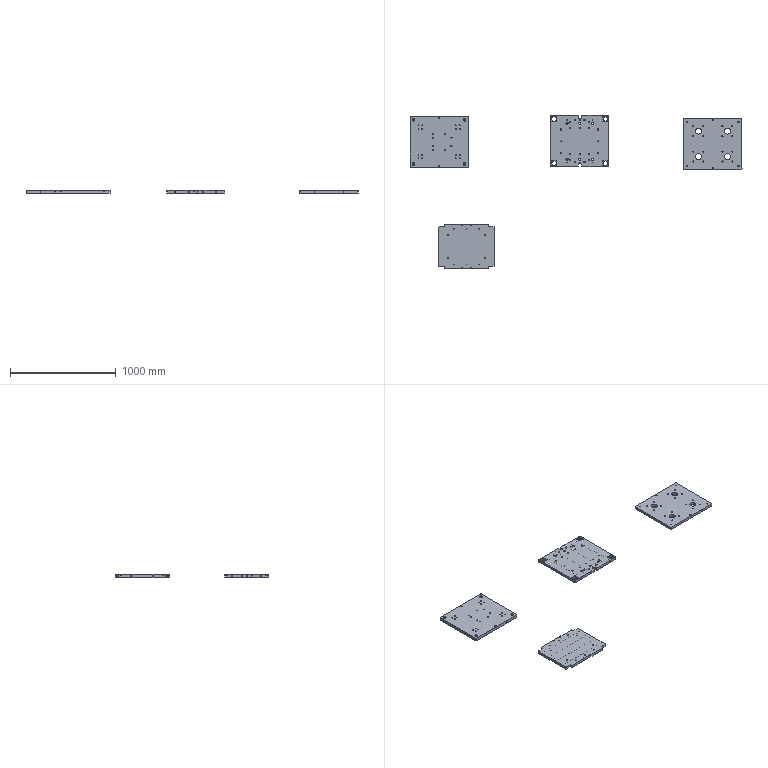NC program | Mastercam | posted with a generic post | part box 3140 x 1452 x 30 mm
Lines 1 to 1913 of 6493, first 1630 of 1913 lines:
%
O0000()
(MATERIAL - ALUMINUM MM - 2024)
( T16 | 16 FEM | H16 | XY STOCK TO LEAVE - .1 | Z STOCK TO LEAVE - .05 )
( T12 | 12 FEM | H12 | XY STOCK TO LEAVE - 0. | Z STOCK TO LEAVE - .05 )
( T7 | 4 CHM | H7 )
( T1 | 11 DR | H1 )
( T2 | 5.5 DR | H2 )
( T3 | 10.5 DR | H3 )
( T5 | 5 FEM | H5 | XY STOCK TO LEAVE - .07 | Z STOCK TO LEAVE - .05 )
( T8 | 8 FEM | H8 | XY STOCK TO LEAVE - .07 | Z STOCK TO LEAVE - .05 )
( T15 | 5.2 DR | H15 )
N100 G21
N110 G0 G17 G40 G49 G80 G90
( ? )
N120 T16 M6
N130 G0 G90 G54 X283.1 Y253.5 A0. S6000 M3
N140 G43 H16 Z50. M8
N150 Z1.2
N160 G1 Z-.294 F600.
N170 Y237.5 F4000.
N180 Y-237.5
N190 Y-253.5
N200 Z-.789 F600.
N210 Y-237.5 F4000.
N220 Y237.5
N230 Y253.5
N240 Z-1.283 F600.
N250 Y237.5 F4000.
N260 Y-237.5
N270 Y-253.5
N280 Z-1.777 F600.
N290 Y-237.5 F4000.
N300 Y237.5
N310 Y253.5
N320 Z-2.271 F600.
N330 Y237.5 F4000.
N340 Y-237.5
N350 Y-253.5
N360 Z-2.766 F600.
N370 Y-237.5 F4000.
N380 Y237.5
N390 Y253.5
N400 Z-3.26 F600.
N410 Y237.5 F4000.
N420 Y-237.5
N430 Y-253.5
N440 Z-3.754 F600.
N450 Y-237.5 F4000.
N460 Y237.5
N470 Y253.5
N480 Z-4.248 F600.
N490 Y237.5 F4000.
N500 Y-237.5
N510 Y-253.5
N520 Z-4.743 F600.
N530 Y-237.5 F4000.
N540 Y237.5
N550 Y253.5
N560 Z-5.237 F600.
N570 Y237.5 F4000.
N580 Y-237.5
N590 Y-253.5
N600 Z-5.731 F600.
N610 Y-237.5 F4000.
N620 Y237.5
N630 Y253.5
N640 Z-6.225 F600.
N650 Y237.5 F4000.
N660 Y-237.5
N670 Y-253.5
N680 Z-6.72 F600.
N690 Y-237.5 F4000.
N700 Y237.5
N710 Y253.5
N720 Z-7.214 F600.
N730 Y237.5 F4000.
N740 Y-237.5
N750 Y-253.5
N760 Z-7.708 F600.
N770 Y-237.5 F4000.
N780 Y237.5
N790 Y253.5
N800 Z-8.202 F600.
N810 Y237.5 F4000.
N820 Y-237.5
N830 Y-253.5
N840 Z-8.697 F600.
N850 Y-237.5 F4000.
N860 Y237.5
N870 Y253.5
N880 Z-9.191 F600.
N890 Y237.5 F4000.
N900 Y-237.5
N910 Y-253.5
N920 Z-9.685 F600.
N930 Y-237.5 F4000.
N940 Y237.5
N950 Y253.5
N960 Z-10.18 F600.
N970 Y237.5 F4000.
N980 Y-237.5
N990 Y-253.5
N1000 Z-10.674 F600.
N1010 Y-237.5 F4000.
N1020 Y237.5
N1030 Y253.5
N1040 Z-11.168 F600.
N1050 Y237.5 F4000.
N1060 Y-237.5
N1070 Y-253.5
N1080 Z-11.662 F600.
N1090 Y-237.5 F4000.
N1100 Y237.5
N1110 Y253.5
N1120 Z-12.157 F600.
N1130 Y237.5 F4000.
N1140 Y-237.5
N1150 Y-253.5
N1160 Z-12.651 F600.
N1170 Y-237.5 F4000.
N1180 Y237.5
N1190 Y253.5
N1200 Z-13.145 F600.
N1210 Y237.5 F4000.
N1220 Y-237.5
N1230 Y-253.5
N1240 Z-13.639 F600.
N1250 Y-237.5 F4000.
N1260 Y237.5
N1270 Y253.5
N1280 Z-14.134 F600.
N1290 Y237.5 F4000.
N1300 Y-237.5
N1310 Y-253.5
N1320 Z-14.628 F600.
N1330 Y-237.5 F4000.
N1340 Y237.5
N1350 Y253.5
N1360 Z-15.122 F600.
N1370 Y237.5 F4000.
N1380 Y-237.5
N1390 Y-253.5
N1400 Z-15.616 F600.
N1410 Y-237.5 F4000.
N1420 Y237.5
N1430 Y253.5
N1440 Z-16.111 F600.
N1450 Y237.5 F4000.
N1460 Y-237.5
N1470 Y-253.5
N1480 Z-16.605 F600.
N1490 Y-237.5 F4000.
N1500 Y237.5
N1510 Y253.5
N1520 Z-17.099 F600.
N1530 Y237.5 F4000.
N1540 Y-237.5
N1550 Y-253.5
N1560 Z-17.593 F600.
N1570 Y-237.5 F4000.
N1580 Y237.5
N1590 Y253.5
N1600 Z-18.088 F600.
N1610 Y237.5 F4000.
N1620 Y-237.5
N1630 Y-253.5
N1640 Z-18.582 F600.
N1650 Y-237.5 F4000.
N1660 Y237.5
N1670 Y253.5
N1680 Z-19.076 F600.
N1690 Y237.5 F4000.
N1700 Y-237.5
N1710 Y-253.5
N1720 Z-19.57 F600.
N1730 Y-237.5 F4000.
N1740 Y237.5
N1750 Y253.5
N1760 Z-20.065 F600.
N1770 Y237.5 F4000.
N1780 Y-237.5
N1790 Y-253.5
N1800 Z-20.559 F600.
N1810 Y-237.5 F4000.
N1820 Y237.5
N1830 Y253.5
N1840 Z-21.053 F600.
N1850 Y237.5 F4000.
N1860 Y-237.5
N1870 Y-253.5
N1880 Z-21.548 F600.
N1890 Y-237.5 F4000.
N1900 Y237.5
N1910 Y253.5
N1920 Z-22.042 F600.
N1930 Y237.5 F4000.
N1940 Y-237.5
N1950 Y-253.5
N1960 Z-22.536 F600.
N1970 Y-237.5 F4000.
N1980 Y237.5
N1990 Y253.5
N2000 Z-23.03 F600.
N2010 Y237.5 F4000.
N2020 Y-237.5
N2030 Y-253.5
N2040 Z-23.525 F600.
N2050 Y-237.5 F4000.
N2060 Y237.5
N2070 Y253.5
N2080 Z-24.019 F600.
N2090 Y237.5 F4000.
N2100 Y-237.5
N2110 Y-253.5
N2120 Z-24.513 F600.
N2130 Y-237.5 F4000.
N2140 Y237.5
N2150 Y253.5
N2160 Z-25.007 F600.
N2170 Y237.5 F4000.
N2180 Y-237.5
N2190 Y-253.5
N2200 Z-25.502 F600.
N2210 Y-237.5 F4000.
N2220 Y237.5
N2230 Y253.5
N2240 Z-25.996 F600.
N2250 Y237.5 F4000.
N2260 Y-237.5
N2270 Y-253.5
N2280 Z-26.49 F600.
N2290 Y-237.5 F4000.
N2300 Y237.5
N2310 Y253.5
N2320 Z-26.984 F600.
N2330 Y237.5 F4000.
N2340 Y-237.5
N2350 Y-253.5
N2360 Z-27.479 F600.
N2370 Y-237.5 F4000.
N2380 Y237.5
N2390 Y253.5
N2400 Z-27.973 F600.
N2410 Y237.5 F4000.
N2420 Y-237.5
N2430 Y-253.5
N2440 Z-28.467 F600.
N2450 Y-237.5 F4000.
N2460 Y237.5
N2470 Y253.5
N2480 Z-28.961 F600.
N2490 Y237.5 F4000.
N2500 Y-237.5
N2510 Y-253.5
N2520 Z-29.456 F600.
N2530 Y-237.5 F4000.
N2540 Y237.5
N2550 Y253.5
N2560 Z-29.95 F600.
N2570 Y237.5 F4000.
N2580 Y-237.5
N2590 Y-253.5
N2600 G0 Z50.
N2610 X-283.1
N2620 Z1.2
N2630 G1 Z-.294 F600.
N2640 Y-237.5 F4000.
N2650 Y237.5
N2660 Y253.5
N2670 Z-.789 F600.
N2680 Y237.5 F4000.
N2690 Y-237.5
N2700 Y-253.5
N2710 Z-1.283 F600.
N2720 Y-237.5 F4000.
N2730 Y237.5
N2740 Y253.5
N2750 Z-1.777 F600.
N2760 Y237.5 F4000.
N2770 Y-237.5
N2780 Y-253.5
N2790 Z-2.271 F600.
N2800 Y-237.5 F4000.
N2810 Y237.5
N2820 Y253.5
N2830 Z-2.766 F600.
N2840 Y237.5 F4000.
N2850 Y-237.5
N2860 Y-253.5
N2870 Z-3.26 F600.
N2880 Y-237.5 F4000.
N2890 Y237.5
N2900 Y253.5
N2910 Z-3.754 F600.
N2920 Y237.5 F4000.
N2930 Y-237.5
N2940 Y-253.5
N2950 Z-4.248 F600.
N2960 Y-237.5 F4000.
N2970 Y237.5
N2980 Y253.5
N2990 Z-4.743 F600.
N3000 Y237.5 F4000.
N3010 Y-237.5
N3020 Y-253.5
N3030 Z-5.237 F600.
N3040 Y-237.5 F4000.
N3050 Y237.5
N3060 Y253.5
N3070 Z-5.731 F600.
N3080 Y237.5 F4000.
N3090 Y-237.5
N3100 Y-253.5
N3110 Z-6.225 F600.
N3120 Y-237.5 F4000.
N3130 Y237.5
N3140 Y253.5
N3150 Z-6.72 F600.
N3160 Y237.5 F4000.
N3170 Y-237.5
N3180 Y-253.5
N3190 Z-7.214 F600.
N3200 Y-237.5 F4000.
N3210 Y237.5
N3220 Y253.5
N3230 Z-7.708 F600.
N3240 Y237.5 F4000.
N3250 Y-237.5
N3260 Y-253.5
N3270 Z-8.202 F600.
N3280 Y-237.5 F4000.
N3290 Y237.5
N3300 Y253.5
N3310 Z-8.697 F600.
N3320 Y237.5 F4000.
N3330 Y-237.5
N3340 Y-253.5
N3350 Z-9.191 F600.
N3360 Y-237.5 F4000.
N3370 Y237.5
N3380 Y253.5
N3390 Z-9.685 F600.
N3400 Y237.5 F4000.
N3410 Y-237.5
N3420 Y-253.5
N3430 Z-10.18 F600.
N3440 Y-237.5 F4000.
N3450 Y237.5
N3460 Y253.5
N3470 Z-10.674 F600.
N3480 Y237.5 F4000.
N3490 Y-237.5
N3500 Y-253.5
N3510 Z-11.168 F600.
N3520 Y-237.5 F4000.
N3530 Y237.5
N3540 Y253.5
N3550 Z-11.662 F600.
N3560 Y237.5 F4000.
N3570 Y-237.5
N3580 Y-253.5
N3590 Z-12.157 F600.
N3600 Y-237.5 F4000.
N3610 Y237.5
N3620 Y253.5
N3630 Z-12.651 F600.
N3640 Y237.5 F4000.
N3650 Y-237.5
N3660 Y-253.5
N3670 Z-13.145 F600.
N3680 Y-237.5 F4000.
N3690 Y237.5
N3700 Y253.5
N3710 Z-13.639 F600.
N3720 Y237.5 F4000.
N3730 Y-237.5
N3740 Y-253.5
N3750 Z-14.134 F600.
N3760 Y-237.5 F4000.
N3770 Y237.5
N3780 Y253.5
N3790 Z-14.628 F600.
N3800 Y237.5 F4000.
N3810 Y-237.5
N3820 Y-253.5
N3830 Z-15.122 F600.
N3840 Y-237.5 F4000.
N3850 Y237.5
N3860 Y253.5
N3870 Z-15.616 F600.
N3880 Y237.5 F4000.
N3890 Y-237.5
N3900 Y-253.5
N3910 Z-16.111 F600.
N3920 Y-237.5 F4000.
N3930 Y237.5
N3940 Y253.5
N3950 Z-16.605 F600.
N3960 Y237.5 F4000.
N3970 Y-237.5
N3980 Y-253.5
N3990 Z-17.099 F600.
N4000 Y-237.5 F4000.
N4010 Y237.5
N4020 Y253.5
N4030 Z-17.593 F600.
N4040 Y237.5 F4000.
N4050 Y-237.5
N4060 Y-253.5
N4070 Z-18.088 F600.
N4080 Y-237.5 F4000.
N4090 Y237.5
N4100 Y253.5
N4110 Z-18.582 F600.
N4120 Y237.5 F4000.
N4130 Y-237.5
N4140 Y-253.5
N4150 Z-19.076 F600.
N4160 Y-237.5 F4000.
N4170 Y237.5
N4180 Y253.5
N4190 Z-19.57 F600.
N4200 Y237.5 F4000.
N4210 Y-237.5
N4220 Y-253.5
N4230 Z-20.065 F600.
N4240 Y-237.5 F4000.
N4250 Y237.5
N4260 Y253.5
N4270 Z-20.559 F600.
N4280 Y237.5 F4000.
N4290 Y-237.5
N4300 Y-253.5
N4310 Z-21.053 F600.
N4320 Y-237.5 F4000.
N4330 Y237.5
N4340 Y253.5
N4350 Z-21.548 F600.
N4360 Y237.5 F4000.
N4370 Y-237.5
N4380 Y-253.5
N4390 Z-22.042 F600.
N4400 Y-237.5 F4000.
N4410 Y237.5
N4420 Y253.5
N4430 Z-22.536 F600.
N4440 Y237.5 F4000.
N4450 Y-237.5
N4460 Y-253.5
N4470 Z-23.03 F600.
N4480 Y-237.5 F4000.
N4490 Y237.5
N4500 Y253.5
N4510 Z-23.525 F600.
N4520 Y237.5 F4000.
N4530 Y-237.5
N4540 Y-253.5
N4550 Z-24.019 F600.
N4560 Y-237.5 F4000.
N4570 Y237.5
N4580 Y253.5
N4590 Z-24.513 F600.
N4600 Y237.5 F4000.
N4610 Y-237.5
N4620 Y-253.5
N4630 Z-25.007 F600.
N4640 Y-237.5 F4000.
N4650 Y237.5
N4660 Y253.5
N4670 Z-25.502 F600.
N4680 Y237.5 F4000.
N4690 Y-237.5
N4700 Y-253.5
N4710 Z-25.996 F600.
N4720 Y-237.5 F4000.
N4730 Y237.5
N4740 Y253.5
N4750 Z-26.49 F600.
N4760 Y237.5 F4000.
N4770 Y-237.5
N4780 Y-253.5
N4790 Z-26.984 F600.
N4800 Y-237.5 F4000.
N4810 Y237.5
N4820 Y253.5
N4830 Z-27.479 F600.
N4840 Y237.5 F4000.
N4850 Y-237.5
N4860 Y-253.5
N4870 Z-27.973 F600.
N4880 Y-237.5 F4000.
N4890 Y237.5
N4900 Y253.5
N4910 Z-28.467 F600.
N4920 Y237.5 F4000.
N4930 Y-237.5
N4940 Y-253.5
N4950 Z-28.961 F600.
N4960 Y-237.5 F4000.
N4970 Y237.5
N4980 Y253.5
N4990 Z-29.456 F600.
N5000 Y237.5 F4000.
N5010 Y-237.5
N5020 Y-253.5
N5030 Z-29.95 F600.
N5040 Y-237.5 F4000.
N5050 Y237.5
N5060 Y253.5
N5070 G0 Z50.
N5080 M5
N5090 G91 G28 Z0. M9
N5100 A0.
N5110 M01
N5120 T12 M6
N5130 G0 G90 G17 G54 X281. Y249.5 A0. S6000 M3
N5140 G43 H12 Z50. M8
N5150 Z1.2
N5160 G1 Z-14.875 F600.
N5170 Y237.5 F1000.
N5180 Y-237.5
N5190 Y-249.5
N5200 G0 Z50.
N5210 Y249.5
N5220 Z-13.875
N5230 G1 Z-29.95 F600.
N5240 Y237.5 F1000.
N5250 Y-237.5
N5260 Y-249.5
N5270 G0 Z50.
N5280 X-281.
N5290 Z1.2
N5300 G1 Z-14.875 F600.
N5310 Y-237.5 F1000.
N5320 Y237.5
N5330 Y249.5
N5340 G0 Z50.
N5350 Y-249.5
N5360 Z-13.875
N5370 G1 Z-29.95 F600.
N5380 Y-237.5 F1000.
N5390 Y237.5
N5400 Y249.5
N5410 G0 Z50.
N5420 M5
N5430 G91 G28 Z0. M9
N5440 A0.
N5450 M01
N5460 T7 M6
N5470 G0 G90 G17 G54 X275.65 Y243.5 A0. S6000 M3
N5480 G43 H7 Z50. M8
N5490 Z1.2
N5500 G1 Z-.75 F600.
N5510 Y237.5 F1000.
N5520 Y-237.5
N5530 Y-243.5
N5540 G0 Z50.
N5550 X-275.65
N5560 Z1.2
N5570 G1 Z-.75 F600.
N5580 Y-237.5 F1000.
N5590 Y237.5
N5600 Y243.5
N5610 G0 Z50.
N5620 M5
N5630 G91 G28 Z0. M9
N5640 A0.
N5650 M01
( ?X )
M00
N5660 T16 M6
N5670 G0 G90 G17 G54 X286.3 Y-235.9 A0. S6000 M3
N5680 G43 H16 Z50. M8
N5690 Z1.2
N5700 G1 Z-.485 F600.
N5710 X284.7 F4000.
N5720 G3 X283.1 Y-237.5 I0. J-1.6
N5730 G2 X270. Y-250.6 I-13.1 J0.
N5740 G1 X-270.
N5750 G2 X-283.1 Y-237.5 I0. J13.1
N5760 G3 X-284.7 Y-235.9 I-1.6 J0.
N5770 G1 X-286.3
N5780 Z-1.17 F600.
N5790 X-284.7 F4000.
N5800 G2 X-283.1 Y-237.5 I0. J-1.6
N5810 G3 X-270. Y-250.6 I13.1 J0.
N5820 G1 X270.
N5830 G3 X283.1 Y-237.5 I0. J13.1
N5840 G2 X284.7 Y-235.9 I1.6 J0.
N5850 G1 X286.3
N5860 Z-1.856 F600.
N5870 X284.7 F4000.
N5880 G3 X283.1 Y-237.5 I0. J-1.6
N5890 G2 X270. Y-250.6 I-13.1 J0.
N5900 G1 X-270.
N5910 G2 X-283.1 Y-237.5 I0. J13.1
N5920 G3 X-284.7 Y-235.9 I-1.6 J0.
N5930 G1 X-286.3
N5940 Z-2.541 F600.
N5950 X-284.7 F4000.
N5960 G2 X-283.1 Y-237.5 I0. J-1.6
N5970 G3 X-270. Y-250.6 I13.1 J0.
N5980 G1 X270.
N5990 G3 X283.1 Y-237.5 I0. J13.1
N6000 G2 X284.7 Y-235.9 I1.6 J0.
N6010 G1 X286.3
N6020 Z-3.226 F600.
N6030 X284.7 F4000.
N6040 G3 X283.1 Y-237.5 I0. J-1.6
N6050 G2 X270. Y-250.6 I-13.1 J0.
N6060 G1 X-270.
N6070 G2 X-283.1 Y-237.5 I0. J13.1
N6080 G3 X-284.7 Y-235.9 I-1.6 J0.
N6090 G1 X-286.3
N6100 Z-3.911 F600.
N6110 X-284.7 F4000.
N6120 G2 X-283.1 Y-237.5 I0. J-1.6
N6130 G3 X-270. Y-250.6 I13.1 J0.
N6140 G1 X270.
N6150 G3 X283.1 Y-237.5 I0. J13.1
N6160 G2 X284.7 Y-235.9 I1.6 J0.
N6170 G1 X286.3
N6180 Z-4.597 F600.
N6190 X284.7 F4000.
N6200 G3 X283.1 Y-237.5 I0. J-1.6
N6210 G2 X270. Y-250.6 I-13.1 J0.
N6220 G1 X-270.
N6230 G2 X-283.1 Y-237.5 I0. J13.1
N6240 G3 X-284.7 Y-235.9 I-1.6 J0.
N6250 G1 X-286.3
N6260 Z-5.282 F600.
N6270 X-284.7 F4000.
N6280 G2 X-283.1 Y-237.5 I0. J-1.6
N6290 G3 X-270. Y-250.6 I13.1 J0.
N6300 G1 X270.
N6310 G3 X283.1 Y-237.5 I0. J13.1
N6320 G2 X284.7 Y-235.9 I1.6 J0.
N6330 G1 X286.3
N6340 Z-5.967 F600.
N6350 X284.7 F4000.
N6360 G3 X283.1 Y-237.5 I0. J-1.6
N6370 G2 X270. Y-250.6 I-13.1 J0.
N6380 G1 X-270.
N6390 G2 X-283.1 Y-237.5 I0. J13.1
N6400 G3 X-284.7 Y-235.9 I-1.6 J0.
N6410 G1 X-286.3
N6420 Z-6.652 F600.
N6430 X-284.7 F4000.
N6440 G2 X-283.1 Y-237.5 I0. J-1.6
N6450 G3 X-270. Y-250.6 I13.1 J0.
N6460 G1 X270.
N6470 G3 X283.1 Y-237.5 I0. J13.1
N6480 G2 X284.7 Y-235.9 I1.6 J0.
N6490 G1 X286.3
N6500 Z-7.338 F600.
N6510 X284.7 F4000.
N6520 G3 X283.1 Y-237.5 I0. J-1.6
N6530 G2 X270. Y-250.6 I-13.1 J0.
N6540 G1 X-270.
N6550 G2 X-283.1 Y-237.5 I0. J13.1
N6560 G3 X-284.7 Y-235.9 I-1.6 J0.
N6570 G1 X-286.3
N6580 Z-8.023 F600.
N6590 X-284.7 F4000.
N6600 G2 X-283.1 Y-237.5 I0. J-1.6
N6610 G3 X-270. Y-250.6 I13.1 J0.
N6620 G1 X270.
N6630 G3 X283.1 Y-237.5 I0. J13.1
N6640 G2 X284.7 Y-235.9 I1.6 J0.
N6650 G1 X286.3
N6660 Z-8.708 F600.
N6670 X284.7 F4000.
N6680 G3 X283.1 Y-237.5 I0. J-1.6
N6690 G2 X270. Y-250.6 I-13.1 J0.
N6700 G1 X-270.
N6710 G2 X-283.1 Y-237.5 I0. J13.1
N6720 G3 X-284.7 Y-235.9 I-1.6 J0.
N6730 G1 X-286.3
N6740 Z-9.393 F600.
N6750 X-284.7 F4000.
N6760 G2 X-283.1 Y-237.5 I0. J-1.6
N6770 G3 X-270. Y-250.6 I13.1 J0.
N6780 G1 X270.
N6790 G3 X283.1 Y-237.5 I0. J13.1
N6800 G2 X284.7 Y-235.9 I1.6 J0.
N6810 G1 X286.3
N6820 Z-10.078 F600.
N6830 X284.7 F4000.
N6840 G3 X283.1 Y-237.5 I0. J-1.6
N6850 G2 X270. Y-250.6 I-13.1 J0.
N6860 G1 X-270.
N6870 G2 X-283.1 Y-237.5 I0. J13.1
N6880 G3 X-284.7 Y-235.9 I-1.6 J0.
N6890 G1 X-286.3
N6900 Z-10.764 F600.
N6910 X-284.7 F4000.
N6920 G2 X-283.1 Y-237.5 I0. J-1.6
N6930 G3 X-270. Y-250.6 I13.1 J0.
N6940 G1 X270.
N6950 G3 X283.1 Y-237.5 I0. J13.1
N6960 G2 X284.7 Y-235.9 I1.6 J0.
N6970 G1 X286.3
N6980 Z-11.449 F600.
N6990 X284.7 F4000.
N7000 G3 X283.1 Y-237.5 I0. J-1.6
N7010 G2 X270. Y-250.6 I-13.1 J0.
N7020 G1 X-270.
N7030 G2 X-283.1 Y-237.5 I0. J13.1
N7040 G3 X-284.7 Y-235.9 I-1.6 J0.
N7050 G1 X-286.3
N7060 Z-12.134 F600.
N7070 X-284.7 F4000.
N7080 G2 X-283.1 Y-237.5 I0. J-1.6
N7090 G3 X-270. Y-250.6 I13.1 J0.
N7100 G1 X270.
N7110 G3 X283.1 Y-237.5 I0. J13.1
N7120 G2 X284.7 Y-235.9 I1.6 J0.
N7130 G1 X286.3
N7140 Z-12.819 F600.
N7150 X284.7 F4000.
N7160 G3 X283.1 Y-237.5 I0. J-1.6
N7170 G2 X270. Y-250.6 I-13.1 J0.
N7180 G1 X-270.
N7190 G2 X-283.1 Y-237.5 I0. J13.1
N7200 G3 X-284.7 Y-235.9 I-1.6 J0.
N7210 G1 X-286.3
N7220 Z-13.505 F600.
N7230 X-284.7 F4000.
N7240 G2 X-283.1 Y-237.5 I0. J-1.6
N7250 G3 X-270. Y-250.6 I13.1 J0.
N7260 G1 X270.
N7270 G3 X283.1 Y-237.5 I0. J13.1
N7280 G2 X284.7 Y-235.9 I1.6 J0.
N7290 G1 X286.3
N7300 Z-14.19 F600.
N7310 X284.7 F4000.
N7320 G3 X283.1 Y-237.5 I0. J-1.6
N7330 G2 X270. Y-250.6 I-13.1 J0.
N7340 G1 X-270.
N7350 G2 X-283.1 Y-237.5 I0. J13.1
N7360 G3 X-284.7 Y-235.9 I-1.6 J0.
N7370 G1 X-286.3
N7380 Z-14.875 F600.
N7390 X-284.7 F4000.
N7400 G2 X-283.1 Y-237.5 I0. J-1.6
N7410 G3 X-270. Y-250.6 I13.1 J0.
N7420 G1 X270.
N7430 G3 X283.1 Y-237.5 I0. J13.1
N7440 G2 X284.7 Y-235.9 I1.6 J0.
N7450 G1 X286.3
N7460 Z-15.56 F600.
N7470 X284.7 F4000.
N7480 G3 X283.1 Y-237.5 I0. J-1.6
N7490 G2 X270. Y-250.6 I-13.1 J0.
N7500 G1 X-270.
N7510 G2 X-283.1 Y-237.5 I0. J13.1
N7520 G3 X-284.7 Y-235.9 I-1.6 J0.
N7530 G1 X-286.3
N7540 Z-16.245 F600.
N7550 X-284.7 F4000.
N7560 G2 X-283.1 Y-237.5 I0. J-1.6
N7570 G3 X-270. Y-250.6 I13.1 J0.
N7580 G1 X270.
N7590 G3 X283.1 Y-237.5 I0. J13.1
N7600 G2 X284.7 Y-235.9 I1.6 J0.
N7610 G1 X286.3
N7620 Z-16.931 F600.
N7630 X284.7 F4000.
N7640 G3 X283.1 Y-237.5 I0. J-1.6
N7650 G2 X270. Y-250.6 I-13.1 J0.
N7660 G1 X-270.
N7670 G2 X-283.1 Y-237.5 I0. J13.1
N7680 G3 X-284.7 Y-235.9 I-1.6 J0.
N7690 G1 X-286.3
N7700 Z-17.616 F600.
N7710 X-284.7 F4000.
N7720 G2 X-283.1 Y-237.5 I0. J-1.6
N7730 G3 X-270. Y-250.6 I13.1 J0.
N7740 G1 X270.
N7750 G3 X283.1 Y-237.5 I0. J13.1
N7760 G2 X284.7 Y-235.9 I1.6 J0.
N7770 G1 X286.3
N7780 Z-18.301 F600.
N7790 X284.7 F4000.
N7800 G3 X283.1 Y-237.5 I0. J-1.6
N7810 G2 X270. Y-250.6 I-13.1 J0.
N7820 G1 X-270.
N7830 G2 X-283.1 Y-237.5 I0. J13.1
N7840 G3 X-284.7 Y-235.9 I-1.6 J0.
N7850 G1 X-286.3
N7860 Z-18.986 F600.
N7870 X-284.7 F4000.
N7880 G2 X-283.1 Y-237.5 I0. J-1.6
N7890 G3 X-270. Y-250.6 I13.1 J0.
N7900 G1 X270.
N7910 G3 X283.1 Y-237.5 I0. J13.1
N7920 G2 X284.7 Y-235.9 I1.6 J0.
N7930 G1 X286.3
N7940 Z-19.672 F600.
N7950 X284.7 F4000.
N7960 G3 X283.1 Y-237.5 I0. J-1.6
N7970 G2 X270. Y-250.6 I-13.1 J0.
N7980 G1 X-270.
N7990 G2 X-283.1 Y-237.5 I0. J13.1
N8000 G3 X-284.7 Y-235.9 I-1.6 J0.
N8010 G1 X-286.3
N8020 Z-20.357 F600.
N8030 X-284.7 F4000.
N8040 G2 X-283.1 Y-237.5 I0. J-1.6
N8050 G3 X-270. Y-250.6 I13.1 J0.
N8060 G1 X270.
N8070 G3 X283.1 Y-237.5 I0. J13.1
N8080 G2 X284.7 Y-235.9 I1.6 J0.
N8090 G1 X286.3
N8100 Z-21.042 F600.
N8110 X284.7 F4000.
N8120 G3 X283.1 Y-237.5 I0. J-1.6
N8130 G2 X270. Y-250.6 I-13.1 J0.
N8140 G1 X-270.
N8150 G2 X-283.1 Y-237.5 I0. J13.1
N8160 G3 X-284.7 Y-235.9 I-1.6 J0.
N8170 G1 X-286.3
N8180 Z-21.727 F600.
N8190 X-284.7 F4000.
N8200 G2 X-283.1 Y-237.5 I0. J-1.6
N8210 G3 X-270. Y-250.6 I13.1 J0.
N8220 G1 X270.
N8230 G3 X283.1 Y-237.5 I0. J13.1
N8240 G2 X284.7 Y-235.9 I1.6 J0.
N8250 G1 X286.3
N8260 Z-22.413 F600.
N8270 X284.7 F4000.
N8280 G3 X283.1 Y-237.5 I0. J-1.6
N8290 G2 X270. Y-250.6 I-13.1 J0.
N8300 G1 X-270.
N8310 G2 X-283.1 Y-237.5 I0. J13.1
N8320 G3 X-284.7 Y-235.9 I-1.6 J0.
N8330 G1 X-286.3
N8340 Z-23.098 F600.
N8350 X-284.7 F4000.
N8360 G2 X-283.1 Y-237.5 I0. J-1.6
N8370 G3 X-270. Y-250.6 I13.1 J0.
N8380 G1 X270.
N8390 G3 X283.1 Y-237.5 I0. J13.1
N8400 G2 X284.7 Y-235.9 I1.6 J0.
N8410 G1 X286.3
N8420 Z-23.783 F600.
N8430 X284.7 F4000.
N8440 G3 X283.1 Y-237.5 I0. J-1.6
N8450 G2 X270. Y-250.6 I-13.1 J0.
N8460 G1 X-270.
N8470 G2 X-283.1 Y-237.5 I0. J13.1
N8480 G3 X-284.7 Y-235.9 I-1.6 J0.
N8490 G1 X-286.3
N8500 Z-24.468 F600.
N8510 X-284.7 F4000.
N8520 G2 X-283.1 Y-237.5 I0. J-1.6
N8530 G3 X-270. Y-250.6 I13.1 J0.
N8540 G1 X270.
N8550 G3 X283.1 Y-237.5 I0. J13.1
N8560 G2 X284.7 Y-235.9 I1.6 J0.
N8570 G1 X286.3
N8580 Z-25.153 F600.
N8590 X284.7 F4000.
N8600 G3 X283.1 Y-237.5 I0. J-1.6
N8610 G2 X270. Y-250.6 I-13.1 J0.
N8620 G1 X-270.
N8630 G2 X-283.1 Y-237.5 I0. J13.1
N8640 G3 X-284.7 Y-235.9 I-1.6 J0.
N8650 G1 X-286.3
N8660 Z-25.839 F600.
N8670 X-284.7 F4000.
N8680 G2 X-283.1 Y-237.5 I0. J-1.6
N8690 G3 X-270. Y-250.6 I13.1 J0.
N8700 G1 X270.
N8710 G3 X283.1 Y-237.5 I0. J13.1
N8720 G2 X284.7 Y-235.9 I1.6 J0.
N8730 G1 X286.3
N8740 Z-26.524 F600.
N8750 X284.7 F4000.
N8760 G3 X283.1 Y-237.5 I0. J-1.6
N8770 G2 X270. Y-250.6 I-13.1 J0.
N8780 G1 X-270.
N8790 G2 X-283.1 Y-237.5 I0. J13.1
N8800 G3 X-284.7 Y-235.9 I-1.6 J0.
N8810 G1 X-286.3
N8820 Z-27.209 F600.
N8830 X-284.7 F4000.
N8840 G2 X-283.1 Y-237.5 I0. J-1.6
N8850 G3 X-270. Y-250.6 I13.1 J0.
N8860 G1 X270.
N8870 G3 X283.1 Y-237.5 I0. J13.1
N8880 G2 X284.7 Y-235.9 I1.6 J0.
N8890 G1 X286.3
N8900 Z-27.894 F600.
N8910 X284.7 F4000.
N8920 G3 X283.1 Y-237.5 I0. J-1.6
N8930 G2 X270. Y-250.6 I-13.1 J0.
N8940 G1 X-270.
N8950 G2 X-283.1 Y-237.5 I0. J13.1
N8960 G3 X-284.7 Y-235.9 I-1.6 J0.
N8970 G1 X-286.3
N8980 Z-28.58 F600.
N8990 X-284.7 F4000.
N9000 G2 X-283.1 Y-237.5 I0. J-1.6
N9010 G3 X-270. Y-250.6 I13.1 J0.
N9020 G1 X270.
N9030 G3 X283.1 Y-237.5 I0. J13.1
N9040 G2 X284.7 Y-235.9 I1.6 J0.
N9050 G1 X286.3
N9060 Z-29.265 F600.
N9070 X284.7 F4000.
N9080 G3 X283.1 Y-237.5 I0. J-1.6
N9090 G2 X270. Y-250.6 I-13.1 J0.
N9100 G1 X-270.
N9110 G2 X-283.1 Y-237.5 I0. J13.1
N9120 G3 X-284.7 Y-235.9 I-1.6 J0.
N9130 G1 X-286.3
N9140 Z-29.95 F600.
N9150 X-284.7 F4000.
N9160 G2 X-283.1 Y-237.5 I0. J-1.6
N9170 G3 X-270. Y-250.6 I13.1 J0.
N9180 G1 X270.
N9190 G3 X283.1 Y-237.5 I0. J13.1
N9200 G2 X284.7 Y-235.9 I1.6 J0.
N9210 G1 X286.3
N9220 G0 Z50.
N9230 X-286.3 Y235.9
N9240 Z1.2
N9250 G1 Z-.485 F600.
N9260 X-284.7 F4000.
N9270 G3 X-283.1 Y237.5 I0. J1.6
N9280 G2 X-270. Y250.6 I13.1 J0.
N9290 G1 X270.
N9300 G2 X283.1 Y237.5 I0. J-13.1
N9310 G3 X284.7 Y235.9 I1.6 J0.
N9320 G1 X286.3
N9330 Z-1.17 F600.
N9340 X284.7 F4000.
N9350 G2 X283.1 Y237.5 I0. J1.6
N9360 G3 X270. Y250.6 I-13.1 J0.
N9370 G1 X-270.
N9380 G3 X-283.1 Y237.5 I0. J-13.1
N9390 G2 X-284.7 Y235.9 I-1.6 J0.
N9400 G1 X-286.3
N9410 Z-1.856 F600.
N9420 X-284.7 F4000.
N9430 G3 X-283.1 Y237.5 I0. J1.6
N9440 G2 X-270. Y250.6 I13.1 J0.
N9450 G1 X270.
N9460 G2 X283.1 Y237.5 I0. J-13.1
N9470 G3 X284.7 Y235.9 I1.6 J0.
N9480 G1 X286.3
N9490 Z-2.541 F600.
N9500 X284.7 F4000.
N9510 G2 X283.1 Y237.5 I0. J1.6
N9520 G3 X270. Y250.6 I-13.1 J0.
N9530 G1 X-270.
N9540 G3 X-283.1 Y237.5 I0. J-13.1
N9550 G2 X-284.7 Y235.9 I-1.6 J0.
N9560 G1 X-286.3
N9570 Z-3.226 F600.
N9580 X-284.7 F4000.
N9590 G3 X-283.1 Y237.5 I0. J1.6
N9600 G2 X-270. Y250.6 I13.1 J0.
N9610 G1 X270.
N9620 G2 X283.1 Y237.5 I0. J-13.1
N9630 G3 X284.7 Y235.9 I1.6 J0.
N9640 G1 X286.3
N9650 Z-3.911 F600.
N9660 X284.7 F4000.
N9670 G2 X283.1 Y237.5 I0. J1.6
N9680 G3 X270. Y250.6 I-13.1 J0.
N9690 G1 X-270.
N9700 G3 X-283.1 Y237.5 I0. J-13.1
N9710 G2 X-284.7 Y235.9 I-1.6 J0.
N9720 G1 X-286.3
N9730 Z-4.597 F600.
N9740 X-284.7 F4000.
N9750 G3 X-283.1 Y237.5 I0. J1.6
N9760 G2 X-270. Y250.6 I13.1 J0.
N9770 G1 X270.
N9780 G2 X283.1 Y237.5 I0. J-13.1
N9790 G3 X284.7 Y235.9 I1.6 J0.
N9800 G1 X286.3
N9810 Z-5.282 F600.
N9820 X284.7 F4000.
N9830 G2 X283.1 Y237.5 I0. J1.6
N9840 G3 X270. Y250.6 I-13.1 J0.
N9850 G1 X-270.
N9860 G3 X-283.1 Y237.5 I0. J-13.1
N9870 G2 X-284.7 Y235.9 I-1.6 J0.
N9880 G1 X-286.3
N9890 Z-5.967 F600.
N9900 X-284.7 F4000.
N9910 G3 X-283.1 Y237.5 I0. J1.6
N9920 G2 X-270. Y250.6 I13.1 J0.
N9930 G1 X270.
N9940 G2 X283.1 Y237.5 I0. J-13.1
N9950 G3 X284.7 Y235.9 I1.6 J0.
N9960 G1 X286.3
N9970 Z-6.652 F600.
N9980 X284.7 F4000.
N9990 G2 X283.1 Y237.5 I0. J1.6
N100 G3 X270. Y250.6 I-13.1 J0.
N110 G1 X-270.
N120 G3 X-283.1 Y237.5 I0. J-13.1
N130 G2 X-284.7 Y235.9 I-1.6 J0.
N140 G1 X-286.3
N150 Z-7.338 F600.
N160 X-284.7 F4000.
N170 G3 X-283.1 Y237.5 I0. J1.6
N180 G2 X-270. Y250.6 I13.1 J0.
N190 G1 X270.
N200 G2 X283.1 Y237.5 I0. J-13.1
N210 G3 X284.7 Y235.9 I1.6 J0.
N220 G1 X286.3
N230 Z-8.023 F600.
N240 X284.7 F4000.
N250 G2 X283.1 Y237.5 I0. J1.6
N260 G3 X270. Y250.6 I-13.1 J0.
N270 G1 X-270.
N280 G3 X-283.1 Y237.5 I0. J-13.1
N290 G2 X-284.7 Y235.9 I-1.6 J0.
N300 G1 X-286.3
N310 Z-8.708 F600.
N320 X-284.7 F4000.
N330 G3 X-283.1 Y237.5 I0. J1.6
N340 G2 X-270. Y250.6 I13.1 J0.
N350 G1 X270.
N360 G2 X283.1 Y237.5 I0. J-13.1
N370 G3 X284.7 Y235.9 I1.6 J0.
N380 G1 X286.3
N390 Z-9.393 F600.
N400 X284.7 F4000.
N410 G2 X283.1 Y237.5 I0. J1.6
N420 G3 X270. Y250.6 I-13.1 J0.
N430 G1 X-270.
N440 G3 X-283.1 Y237.5 I0. J-13.1
N450 G2 X-284.7 Y235.9 I-1.6 J0.
N460 G1 X-286.3
N470 Z-10.078 F600.
N480 X-284.7 F4000.
N490 G3 X-283.1 Y237.5 I0. J1.6
N500 G2 X-270. Y250.6 I13.1 J0.
N510 G1 X270.
N520 G2 X283.1 Y237.5 I0. J-13.1
N530 G3 X284.7 Y235.9 I1.6 J0.
N540 G1 X286.3
N550 Z-10.764 F600.
N560 X284.7 F4000.
N570 G2 X283.1 Y237.5 I0. J1.6
N580 G3 X270. Y250.6 I-13.1 J0.
N590 G1 X-270.
N600 G3 X-283.1 Y237.5 I0. J-13.1
N610 G2 X-284.7 Y235.9 I-1.6 J0.
N620 G1 X-286.3
N630 Z-11.449 F600.
N640 X-284.7 F4000.
N650 G3 X-283.1 Y237.5 I0. J1.6
N660 G2 X-270. Y250.6 I13.1 J0.
N670 G1 X270.
N680 G2 X283.1 Y237.5 I0. J-13.1
N690 G3 X284.7 Y235.9 I1.6 J0.
N700 G1 X286.3
N710 Z-12.134 F600.
N720 X284.7 F4000.
N730 G2 X283.1 Y237.5 I0. J1.6
N740 G3 X270. Y250.6 I-13.1 J0.
N750 G1 X-270.
N760 G3 X-283.1 Y237.5 I0. J-13.1
N770 G2 X-284.7 Y235.9 I-1.6 J0.
N780 G1 X-286.3
N790 Z-12.819 F600.
N800 X-284.7 F4000.
N810 G3 X-283.1 Y237.5 I0. J1.6
N820 G2 X-270. Y250.6 I13.1 J0.
N830 G1 X270.
N840 G2 X283.1 Y237.5 I0. J-13.1
N850 G3 X284.7 Y235.9 I1.6 J0.
N860 G1 X286.3
N870 Z-13.505 F600.
N880 X284.7 F4000.
N890 G2 X283.1 Y237.5 I0. J1.6
N900 G3 X270. Y250.6 I-13.1 J0.
N910 G1 X-270.
N920 G3 X-283.1 Y237.5 I0. J-13.1
N930 G2 X-284.7 Y235.9 I-1.6 J0.
N940 G1 X-286.3
N950 Z-14.19 F600.
N960 X-284.7 F4000.
N970 G3 X-283.1 Y237.5 I0. J1.6
N980 G2 X-270. Y250.6 I13.1 J0.
N990 G1 X270.
N1000 G2 X283.1 Y237.5 I0. J-13.1
N1010 G3 X284.7 Y235.9 I1.6 J0.
N1020 G1 X286.3
N1030 Z-14.875 F600.
N1040 X284.7 F4000.
N1050 G2 X283.1 Y237.5 I0. J1.6
N1060 G3 X270. Y250.6 I-13.1 J0.
N1070 G1 X-270.
N1080 G3 X-283.1 Y237.5 I0. J-13.1
N1090 G2 X-284.7 Y235.9 I-1.6 J0.
N1100 G1 X-286.3
N1110 Z-15.56 F600.
N1120 X-284.7 F4000.
N1130 G3 X-283.1 Y237.5 I0. J1.6
N1140 G2 X-270. Y250.6 I13.1 J0.
N1150 G1 X270.
N1160 G2 X283.1 Y237.5 I0. J-13.1
N1170 G3 X284.7 Y235.9 I1.6 J0.
N1180 G1 X286.3
N1190 Z-16.245 F600.
N1200 X284.7 F4000.
N1210 G2 X283.1 Y237.5 I0. J1.6
N1220 G3 X270. Y250.6 I-13.1 J0.
N1230 G1 X-270.
N1240 G3 X-283.1 Y237.5 I0. J-13.1
N1250 G2 X-284.7 Y235.9 I-1.6 J0.
N1260 G1 X-286.3
N1270 Z-16.931 F600.
N1280 X-284.7 F4000.
N1290 G3 X-283.1 Y237.5 I0. J1.6
N1300 G2 X-270. Y250.6 I13.1 J0.
N1310 G1 X270.
N1320 G2 X283.1 Y237.5 I0. J-13.1
N1330 G3 X284.7 Y235.9 I1.6 J0.
N1340 G1 X286.3
N1350 Z-17.616 F600.
N1360 X284.7 F4000.
N1370 G2 X283.1 Y237.5 I0. J1.6
N1380 G3 X270. Y250.6 I-13.1 J0.
N1390 G1 X-270.
N1400 G3 X-283.1 Y237.5 I0. J-13.1
N1410 G2 X-284.7 Y235.9 I-1.6 J0.
N1420 G1 X-286.3
N1430 Z-18.301 F600.
N1440 X-284.7 F4000.
N1450 G3 X-283.1 Y237.5 I0. J1.6
N1460 G2 X-270. Y250.6 I13.1 J0.
N1470 G1 X270.
N1480 G2 X283.1 Y237.5 I0. J-13.1
N1490 G3 X284.7 Y235.9 I1.6 J0.
N1500 G1 X286.3
N1510 Z-18.986 F600.
N1520 X284.7 F4000.
N1530 G2 X283.1 Y237.5 I0. J1.6
N1540 G3 X270. Y250.6 I-13.1 J0.
N1550 G1 X-270.
N1560 G3 X-283.1 Y237.5 I0. J-13.1
N1570 G2 X-284.7 Y235.9 I-1.6 J0.
N1580 G1 X-286.3
N1590 Z-19.672 F600.
N1600 X-284.7 F4000.
N1610 G3 X-283.1 Y237.5 I0. J1.6
N1620 G2 X-270. Y250.6 I13.1 J0.
N1630 G1 X270.
N1640 G2 X283.1 Y237.5 I0. J-13.1
N1650 G3 X284.7 Y235.9 I1.6 J0.
N1660 G1 X286.3
N1670 Z-20.357 F600.
N1680 X284.7 F4000.
N1690 G2 X283.1 Y237.5 I0. J1.6
N1700 G3 X270. Y250.6 I-13.1 J0.
N1710 G1 X-270.
N1720 G3 X-283.1 Y237.5 I0. J-13.1
N1730 G2 X-284.7 Y235.9 I-1.6 J0.
N1740 G1 X-286.3
N1750 Z-21.042 F600.
N1760 X-284.7 F4000.
N1770 G3 X-283.1 Y237.5 I0. J1.6
N1780 G2 X-270. Y250.6 I13.1 J0.
N1790 G1 X270.
N1800 G2 X283.1 Y237.5 I0. J-13.1
N1810 G3 X284.7 Y235.9 I1.6 J0.
N1820 G1 X286.3
N1830 Z-21.727 F600.
N1840 X284.7 F4000.
N1850 G2 X283.1 Y237.5 I0. J1.6
N1860 G3 X270. Y250.6 I-13.1 J0.
N1870 G1 X-270.
N1880 G3 X-283.1 Y237.5 I0. J-13.1
N1890 G2 X-284.7 Y235.9 I-1.6 J0.
N1900 G1 X-286.3
N1910 Z-22.413 F600.
N1920 X-284.7 F4000.
N1930 G3 X-283.1 Y237.5 I0. J1.6
N1940 G2 X-270. Y250.6 I13.1 J0.
N1950 G1 X270.
N1960 G2 X283.1 Y237.5 I0. J-13.1
N1970 G3 X284.7 Y235.9 I1.6 J0.
N1980 G1 X286.3
N1990 Z-23.098 F600.
N2000 X284.7 F4000.
N2010 G2 X283.1 Y237.5 I0. J1.6
N2020 G3 X270. Y250.6 I-13.1 J0.
N2030 G1 X-270.
N2040 G3 X-283.1 Y237.5 I0. J-13.1
N2050 G2 X-284.7 Y235.9 I-1.6 J0.
N2060 G1 X-286.3
N2070 Z-23.783 F600.
N2080 X-284.7 F4000.
N2090 G3 X-283.1 Y237.5 I0. J1.6
N2100 G2 X-270. Y250.6 I13.1 J0.
N2110 G1 X270.
N2120 G2 X283.1 Y237.5 I0. J-13.1
N2130 G3 X284.7 Y235.9 I1.6 J0.
N2140 G1 X286.3
N2150 Z-24.468 F600.
N2160 X284.7 F4000.
N2170 G2 X283.1 Y237.5 I0. J1.6
N2180 G3 X270. Y250.6 I-13.1 J0.
N2190 G1 X-270.
N2200 G3 X-283.1 Y237.5 I0. J-13.1
N2210 G2 X-284.7 Y235.9 I-1.6 J0.
N2220 G1 X-286.3
N2230 Z-25.153 F600.
N2240 X-284.7 F4000.
N2250 G3 X-283.1 Y237.5 I0. J1.6
N2260 G2 X-270. Y250.6 I13.1 J0.
N2270 G1 X270.
N2280 G2 X283.1 Y237.5 I0. J-13.1
N2290 G3 X284.7 Y235.9 I1.6 J0.
N2300 G1 X286.3
N2310 Z-25.839 F600.
N2320 X284.7 F4000.
N2330 G2 X283.1 Y237.5 I0. J1.6
N2340 G3 X270. Y250.6 I-13.1 J0.
N2350 G1 X-270.
N2360 G3 X-283.1 Y237.5 I0. J-13.1
N2370 G2 X-284.7 Y235.9 I-1.6 J0.
N2380 G1 X-286.3
N2390 Z-26.524 F600.
N2400 X-284.7 F4000.
N2410 G3 X-283.1 Y237.5 I0. J1.6
N2420 G2 X-270. Y250.6 I13.1 J0.
N2430 G1 X270.
N2440 G2 X283.1 Y237.5 I0. J-13.1
N2450 G3 X284.7 Y235.9 I1.6 J0.
N2460 G1 X286.3
N2470 Z-27.209 F600.
N2480 X284.7 F4000.
N2490 G2 X283.1 Y237.5 I0. J1.6
N2500 G3 X270. Y250.6 I-13.1 J0.
N2510 G1 X-270.
N2520 G3 X-283.1 Y237.5 I0. J-13.1
N2530 G2 X-284.7 Y235.9 I-1.6 J0.
N2540 G1 X-286.3
N2550 Z-27.894 F600.
N2560 X-284.7 F4000.
N2570 G3 X-283.1 Y237.5 I0. J1.6
N2580 G2 X-270. Y250.6 I13.1 J0.
N2590 G1 X270.
N2600 G2 X283.1 Y237.5 I0. J-13.1
N2610 G3 X284.7 Y235.9 I1.6 J0.
N2620 G1 X286.3
N2630 Z-28.58 F600.
N2640 X284.7 F4000.
N2650 G2 X283.1 Y237.5 I0. J1.6
N2660 G3 X270. Y250.6 I-13.1 J0.
N2670 G1 X-270.
N2680 G3 X-283.1 Y237.5 I0. J-13.1
N2690 G2 X-284.7 Y235.9 I-1.6 J0.
N2700 G1 X-286.3
N2710 Z-29.265 F600.
N2720 X-284.7 F4000.
N2730 G3 X-283.1 Y237.5 I0. J1.6
N2740 G2 X-270. Y250.6 I13.1 J0.
N2750 G1 X270.
N2760 G2 X283.1 Y237.5 I0. J-13.1
N2770 G3 X284.7 Y235.9 I1.6 J0.
N2780 G1 X286.3
N2790 Z-29.95 F600.
N2800 X284.7 F4000.
N2810 G2 X283.1 Y237.5 I0. J1.6
N2820 G3 X270. Y250.6 I-13.1 J0.
N2830 G1 X-270.
N2840 G3 X-283.1 Y237.5 I0. J-13.1
N2850 G2 X-284.7 Y235.9 I-1.6 J0.
N2860 G1 X-286.3
N2870 G0 Z50.
N2880 M5
N2890 G91 G28 Z0. M9
N2900 A0.
N2910 M01
N2920 T12 M6
N2930 G0 G90 G17 G54 X283.4 Y-236.3 A0. S6000 M3
N2940 G43 H12 Z50. M8
N2950 Z1.2
N2960 G1 Z-14.875 F600.
N2970 X282.2 F1000.
N2980 G3 X281. Y-237.5 I0. J-1.2
N2990 G2 X270. Y-248.5 I-11. J0.
N3000 G1 X-270.
N3010 G2 X-281. Y-237.5 I0. J11.
N3020 G3 X-282.2 Y-236.3 I-1.2 J0.
N3030 G1 X-283.4
N3040 G0 Z50.
N3050 X283.4
N3060 Z-13.875
N3070 G1 Z-29.95 F600.
N3080 X282.2 F1000.
N3090 G3 X281. Y-237.5 I0. J-1.2
N3100 G2 X270. Y-248.5 I-11. J0.
N3110 G1 X-270.
N3120 G2 X-281. Y-237.5 I0. J11.
N3130 G3 X-282.2 Y-236.3 I-1.2 J0.
N3140 G1 X-283.4
N3150 G0 Z50.
N3160 Y236.3
N3170 Z1.2
N3180 G1 Z-14.875 F600.
N3190 X-282.2 F1000.
N3200 G3 X-281. Y237.5 I0. J1.2
N3210 G2 X-270. Y248.5 I11. J0.
N3220 G1 X270.
N3230 G2 X281. Y237.5 I0. J-11.
N3240 G3 X282.2 Y236.3 I1.2 J0.
N3250 G1 X283.4
N3260 G0 Z50.
N3270 X-283.4
N3280 Z-13.875
N3290 G1 Z-29.95 F600.
N3300 X-282.2 F1000.
N3310 G3 X-281. Y237.5 I0. J1.2
N3320 G2 X-270. Y248.5 I11. J0.
N3330 G1 X270.
N3340 G2 X281. Y237.5 I0. J-11.
N3350 G3 X282.2 Y236.3 I1.2 J0.
N3360 G1 X283.4
N3370 G0 Z50.
N3380 M5
N3390 G91 G28 Z0. M9
N3400 A0.
N3410 M01
N3420 T7 M6
N3430 G0 G90 G17 G54 X276.45 Y-237.1 A0. S6000 M3
N3440 G43 H7 Z50. M8
N3450 Z1.2
N3460 G1 Z-.75 F600.
N3470 X276.05 F1000.
N3480 G3 X275.65 Y-237.5 I0. J-.4
N3490 G2 X270. Y-243.15 I-5.65 J0.
N3500 G1 X-270.
N3510 G2 X-275.65 Y-237.5 I0. J5.65
N3520 G3 X-276.05 Y-237.1 I-.4 J0.
N3530 G1 X-276.45
N3540 G0 Z50.
N3550 Y237.1
N3560 Z1.2
N3570 G1 Z-.75 F600.
N3580 X-276.05 F1000.
N3590 G3 X-275.65 Y237.5 I0. J.4
N3600 G2 X-270. Y243.15 I5.65 J0.
N3610 G1 X270.
N3620 G2 X275.65 Y237.5 I0. J-5.65
N3630 G3 X276.05 Y237.1 I.4 J0.
N3640 G1 X276.45
N3650 G0 Z50.
N3660 X242. Y-209.
N3670 G98 G81 Z-.7 R1. F200.
N3680 X194.5 Y-156.
N3690 Y-124.
N3700 X158.5 Y-156.
N3710 Y-124.
N3720 X117. Y-40.
N3730 X55. Y-72.5
N3740 X-55.
N3750 X-57. Y-40.
N3760 Y40.
N3770 X-55. Y72.5
N3780 X55.
N3790 X117. Y40.
N3800 X158.5 Y124.
N3810 X194.5
N3820 Y156.
N3830 X242. Y209.
N3840 X158.5 Y156.
N3850 X0. Y227.5
N3860 X-158.5 Y156.
N3870 X-242. Y209.
N3880 X-194.5 Y156.
N3890 Y124.
N3900 X-158.5
N3910 Y-124.
N3920 X-194.5
N3930 Y-156.
N3940 X-242. Y-209.
N3950 X-158.5 Y-156.
N3960 X0. Y-227.5
N3970 G80
N3980 M5
N3990 G91 G0 G28 Z0. M9
N4000 A0.
N4010 M01
N4020 T1 M6
N4030 G0 G90 G17 G54 X242. Y-209. A0. S800 M3
N4040 G43 H1 Z50. M8
N4050 G98 G83 Z-29.8 R1. Q2. F60.
N4060 X0. Y-227.5
N4070 X-242. Y-209.
N4080 Y209.
N4090 X0. Y227.5
N4100 X242. Y209.
N4110 G80
N4120 M5
N4130 G91 G0 G28 Z0. M9
N4140 A0.
N4150 M01
N4160 T2 M6
N4170 G0 G90 G17 G54 X194.5 Y-156. A0. S1200 M3
N4180 G43 H2 Z50. M8
N4190 G98 G83 Z-29.8 R1. Q2. F100.
N4200 X158.5
N4210 Y-124.
N4220 X194.5
N4230 Y124.
N4240 Y156.
N4250 X158.5
N4260 Y124.
N4270 X-158.5
N4280 Y156.
N4290 X-194.5
N4300 Y124.
N4310 Y-124.
N4320 Y-156.
N4330 X-158.5
N4340 Y-124.
N4350 G80
N4360 M5
N4370 G91 G0 G28 Z0. M9
N4380 A0.
N4390 M01
N4400 T3 M6
N4410 G0 G90 G17 G54 X117. Y-40. A0. S800 M3
N4420 G43 H3 Z50. M8
N4430 G98 G83 Z-29.8 R1. Q2. F80.
N4440 X55. Y-72.5
N4450 X-55.
N4460 X-57. Y-40.
N4470 Y40.
N4480 X-55. Y72.5
N4490 X55.
N4500 X117. Y40.
N4510 G80
N4520 M5
N4530 G91 G0 G28 Z0. M9
N4540 A0.
N4550 M01
N4560 T12 M6
N4570 G0 G90 G17 G54 X-238. Y207.8 A0. S7000 M3
N4580 G43 H12 Z50. M8
N4590 Z1.2
N4600 G1 Z.2 F600.
N4610 X-236.8 F3000.
N4620 G3 X-235.6 Y209. I0. J1.2
N4630 X-242. Y215.4 Z.025 I-6.4 J0.
N4640 X-248.4 Y209. Z-.15 I0. J-6.4
N4650 X-242. Y202.6 Z-.325 I6.4 J0.
N4660 X-235.6 Y209. Z-.5 I0. J6.4
N4670 X-242. Y215.4 Z-.675 I-6.4 J0.
N4680 X-248.4 Y209. Z-.85 I0. J-6.4
N4690 X-242. Y202.6 Z-1.025 I6.4 J0.
N4700 X-235.6 Y209. Z-1.2 I0. J6.4
N4710 X-242. Y215.4 Z-1.375 I-6.4 J0.
N4720 X-248.4 Y209. Z-1.55 I0. J-6.4
N4730 X-242. Y202.6 Z-1.725 I6.4 J0.
N4740 X-235.6 Y209. Z-1.9 I0. J6.4
N4750 X-242. Y215.4 Z-2.075 I-6.4 J0.
N4760 X-248.4 Y209. Z-2.25 I0. J-6.4
N4770 X-242. Y202.6 Z-2.425 I6.4 J0.
N4780 X-235.6 Y209. Z-2.6 I0. J6.4
N4790 X-242. Y215.4 Z-2.775 I-6.4 J0.
N4800 X-248.4 Y209. Z-2.95 I0. J-6.4
N4810 X-242. Y202.6 Z-3.125 I6.4 J0.
N4820 X-235.6 Y209. Z-3.3 I0. J6.4
N4830 X-242. Y215.4 Z-3.475 I-6.4 J0.
N4840 X-248.4 Y209. Z-3.65 I0. J-6.4
N4850 X-242. Y202.6 Z-3.825 I6.4 J0.
N4860 X-235.6 Y209. Z-4. I0. J6.4
N4870 X-242. Y215.4 Z-4.175 I-6.4 J0.
N4880 X-248.4 Y209. Z-4.35 I0. J-6.4
N4890 X-242. Y202.6 Z-4.525 I6.4 J0.
N4900 X-235.6 Y209. Z-4.7 I0. J6.4
N4910 X-242. Y215.4 Z-4.875 I-6.4 J0.
N4920 X-248.4 Y209. Z-5.05 I0. J-6.4
N4930 X-242. Y202.6 Z-5.225 I6.4 J0.
N4940 X-235.6 Y209. Z-5.4 I0. J6.4
N4950 X-242. Y215.4 Z-5.575 I-6.4 J0.
N4960 X-248.4 Y209. Z-5.75 I0. J-6.4
N4970 X-242. Y202.6 Z-5.925 I6.4 J0.
N4980 X-235.6 Y209. Z-6.1 I0. J6.4
N4990 X-242. Y215.4 Z-6.275 I-6.4 J0.
N5000 X-248.4 Y209. Z-6.45 I0. J-6.4
N5010 X-242. Y202.6 Z-6.625 I6.4 J0.
N5020 X-235.6 Y209. Z-6.8 I0. J6.4
N5030 X-242. Y215.4 Z-6.975 I-6.4 J0.
N5040 X-248.4 Y209. Z-7.15 I0. J-6.4
N5050 X-242. Y202.6 Z-7.325 I6.4 J0.
N5060 X-235.6 Y209. Z-7.5 I0. J6.4
N5070 X-242. Y215.4 Z-7.675 I-6.4 J0.
N5080 X-248.4 Y209. Z-7.85 I0. J-6.4
N5090 X-242. Y202.6 Z-8.025 I6.4 J0.
N5100 X-235.6 Y209. Z-8.2 I0. J6.4
N5110 X-242. Y215.4 Z-8.375 I-6.4 J0.
N5120 X-248.4 Y209. Z-8.55 I0. J-6.4
N5130 X-242. Y202.6 Z-8.725 I6.4 J0.
N5140 X-235.6 Y209. Z-8.9 I0. J6.4
N5150 X-242. Y215.4 Z-9.075 I-6.4 J0.
N5160 X-248.4 Y209. Z-9.25 I0. J-6.4
N5170 X-242. Y202.6 Z-9.425 I6.4 J0.
N5180 X-235.6 Y209. Z-9.6 I0. J6.4
N5190 X-242. Y215.4 Z-9.775 I-6.4 J0.
N5200 X-248.4 Y209. Z-9.95 I0. J-6.4
N5210 X-242. Y202.6 Z-10.125 I6.4 J0.
N5220 X-235.6 Y209. Z-10.3 I0. J6.4
N5230 X-242. Y215.4 Z-10.475 I-6.4 J0.
N5240 X-248.4 Y209. Z-10.65 I0. J-6.4
N5250 X-242. Y202.6 Z-10.825 I6.4 J0.
N5260 X-235.6 Y209. Z-11. I0. J6.4
N5270 X-242. Y215.4 Z-11.175 I-6.4 J0.
N5280 X-248.4 Y209. Z-11.35 I0. J-6.4
N5290 X-242. Y202.6 Z-11.525 I6.4 J0.
N5300 X-235.6 Y209. Z-11.7 I0. J6.4
N5310 X-242. Y215.4 Z-11.875 I-6.4 J0.
N5320 X-248.4 Y209. Z-12.05 I0. J-6.4
N5330 X-242. Y202.6 Z-12.225 I6.4 J0.
N5340 X-235.6 Y209. Z-12.4 I0. J6.4
N5350 X-242. Y215.4 Z-12.575 I-6.4 J0.
N5360 X-248.4 Y209. Z-12.75 I0. J-6.4
N5370 X-243.424 Y202.76 Z-12.9 I6.4 J0.
N5380 X-242. Y202.6 I1.424 J6.24
N5390 X-235.6 Y209. I0. J6.4
N5400 X-242. Y215.4 I-6.4 J0.
N5410 X-248.4 Y209. I0. J-6.4
N5420 X-242.933 Y202.668 I6.4 J0.
N5430 X-242.758 Y202.655 I.175 J1.188
N5440 X-241.571 Y203.681 I0. J1.201
N5450 G1 X-241.396 Y204.868
N5460 G0 Z50.
N5470 X246. Y207.8
N5480 Z1.2
N5490 G1 Z.2 F600.
N5500 X247.2 F3000.
N5510 G3 X248.4 Y209. I0. J1.2
N5520 X242. Y215.4 Z.025 I-6.4 J0.
N5530 X235.6 Y209. Z-.15 I0. J-6.4
N5540 X242. Y202.6 Z-.325 I6.4 J0.
N5550 X248.4 Y209. Z-.5 I0. J6.4
N5560 X242. Y215.4 Z-.675 I-6.4 J0.
N5570 X235.6 Y209. Z-.85 I0. J-6.4
N5580 X242. Y202.6 Z-1.025 I6.4 J0.
N5590 X248.4 Y209. Z-1.2 I0. J6.4
N5600 X242. Y215.4 Z-1.375 I-6.4 J0.
N5610 X235.6 Y209. Z-1.55 I0. J-6.4
N5620 X242. Y202.6 Z-1.725 I6.4 J0.
N5630 X248.4 Y209. Z-1.9 I0. J6.4
N5640 X242. Y215.4 Z-2.075 I-6.4 J0.
N5650 X235.6 Y209. Z-2.25 I0. J-6.4
N5660 X242. Y202.6 Z-2.425 I6.4 J0.
N5670 X248.4 Y209. Z-2.6 I0. J6.4
N5680 X242. Y215.4 Z-2.775 I-6.4 J0.
N5690 X235.6 Y209. Z-2.95 I0. J-6.4
N5700 X242. Y202.6 Z-3.125 I6.4 J0.
N5710 X248.4 Y209. Z-3.3 I0. J6.4
N5720 X242. Y215.4 Z-3.475 I-6.4 J0.
N5730 X235.6 Y209. Z-3.65 I0. J-6.4
N5740 X242. Y202.6 Z-3.825 I6.4 J0.
N5750 X248.4 Y209. Z-4. I0. J6.4
N5760 X242. Y215.4 Z-4.175 I-6.4 J0.
N5770 X235.6 Y209. Z-4.35 I0. J-6.4
N5780 X242. Y202.6 Z-4.525 I6.4 J0.
N5790 X248.4 Y209. Z-4.7 I0. J6.4
N5800 X242. Y215.4 Z-4.875 I-6.4 J0.
N5810 X235.6 Y209. Z-5.05 I0. J-6.4
N5820 X242. Y202.6 Z-5.225 I6.4 J0.
N5830 X248.4 Y209. Z-5.4 I0. J6.4
N5840 X242. Y215.4 Z-5.575 I-6.4 J0.
N5850 X235.6 Y209. Z-5.75 I0. J-6.4
N5860 X242. Y202.6 Z-5.925 I6.4 J0.
N5870 X248.4 Y209. Z-6.1 I0. J6.4
N5880 X242. Y215.4 Z-6.275 I-6.4 J0.
N5890 X235.6 Y209. Z-6.45 I0. J-6.4
N5900 X242. Y202.6 Z-6.625 I6.4 J0.
N5910 X248.4 Y209. Z-6.8 I0. J6.4
N5920 X242. Y215.4 Z-6.975 I-6.4 J0.
N5930 X235.6 Y209. Z-7.15 I0. J-6.4
N5940 X242. Y202.6 Z-7.325 I6.4 J0.
N5950 X248.4 Y209. Z-7.5 I0. J6.4
N5960 X242. Y215.4 Z-7.675 I-6.4 J0.
N5970 X235.6 Y209. Z-7.85 I0. J-6.4
N5980 X242. Y202.6 Z-8.025 I6.4 J0.
N5990 X248.4 Y209. Z-8.2 I0. J6.4
N6000 X242. Y215.4 Z-8.375 I-6.4 J0.
N6010 X235.6 Y209. Z-8.55 I0. J-6.4
N6020 X242. Y202.6 Z-8.725 I6.4 J0.
N6030 X248.4 Y209. Z-8.9 I0. J6.4
N6040 X242. Y215.4 Z-9.075 I-6.4 J0.
N6050 X235.6 Y209. Z-9.25 I0. J-6.4
N6060 X242. Y202.6 Z-9.425 I6.4 J0.
N6070 X248.4 Y209. Z-9.6 I0. J6.4
N6080 X242. Y215.4 Z-9.775 I-6.4 J0.
N6090 X235.6 Y209. Z-9.95 I0. J-6.4
N6100 X242. Y202.6 Z-10.125 I6.4 J0.
N6110 X248.4 Y209. Z-10.3 I0. J6.4
N6120 X242. Y215.4 Z-10.475 I-6.4 J0.
N6130 X235.6 Y209. Z-10.65 I0. J-6.4
N6140 X242. Y202.6 Z-10.825 I6.4 J0.
N6150 X248.4 Y209. Z-11. I0. J6.4
N6160 X242. Y215.4 Z-11.175 I-6.4 J0.
N6170 X235.6 Y209. Z-11.35 I0. J-6.4
N6180 X242. Y202.6 Z-11.525 I6.4 J0.
N6190 X248.4 Y209. Z-11.7 I0. J6.4
N6200 X242. Y215.4 Z-11.875 I-6.4 J0.
N6210 X235.6 Y209. Z-12.05 I0. J-6.4
N6220 X242. Y202.6 Z-12.225 I6.4 J0.
N6230 X248.4 Y209. Z-12.4 I0. J6.4
N6240 X242. Y215.4 Z-12.575 I-6.4 J0.
N6250 X235.6 Y209. Z-12.75 I0. J-6.4
N6260 X240.576 Y202.76 Z-12.9 I6.4 J0.
N6270 X242. Y202.6 I1.424 J6.24
N6280 X248.4 Y209. I0. J6.4
N6290 X242. Y215.4 I-6.4 J0.
N6300 X235.6 Y209. I0. J-6.4
N6310 X241.067 Y202.668 I6.4 J0.
N6320 X241.242 Y202.655 I.175 J1.188
N6330 X242.429 Y203.681 I0. J1.201
N6340 G1 X242.604 Y204.868